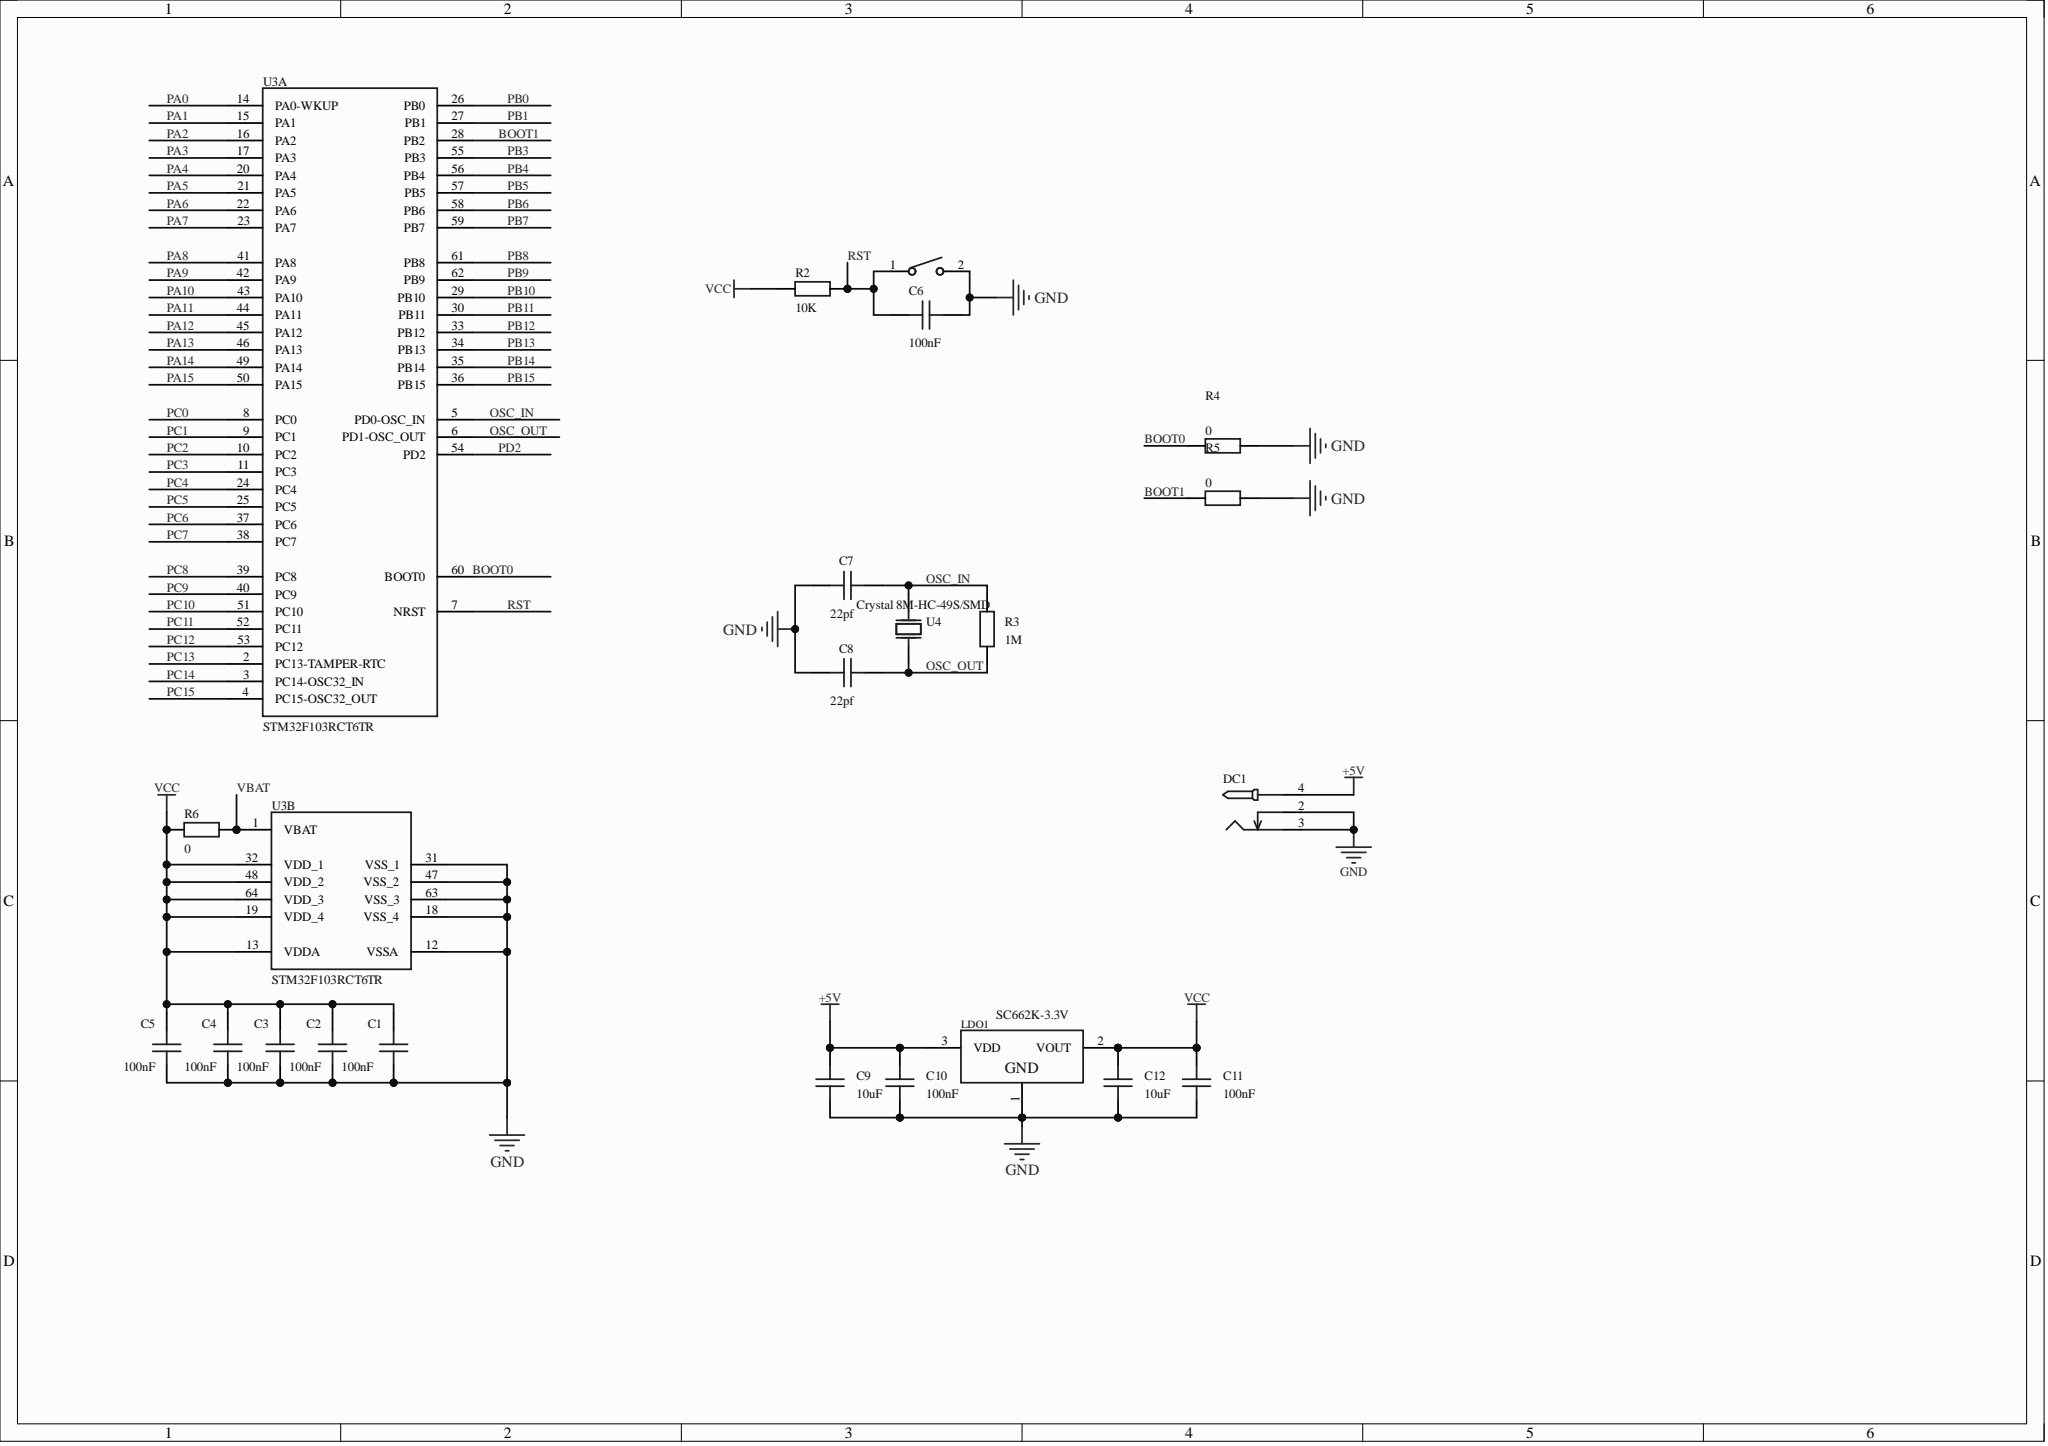Circuit board | Altium Designer | 22 parts | 9 nets
Bill of materials:
Comment,Description,Designator,Footprint,LibRef,Quantity
"100nF","[NoValue], Capacitance:100nF;Tolerance:±10%;Rated voltage:50V;Dielectric (temp. coefficient):X7R;","C1, C2, C3, C4, C5, C6, C10, C11","C0603","CAP_0603, CC0603KRX7R9BB104","8"
"22pf","","C7, C8","C0603","CAP_0603","2"
"10uF","Capacitance:10uF;Tolerance:±10%;Rated voltage:10V;Dielectric (temp. coefficient):X5R;","C9, C12","C0603","CL10A106KP8NNNC","2"
"","","DC1","DC-2.0","DC-005_2.0","1"
"SC662K-3.3V","Output type:Fixed;Output polarity:Positive;Max input voltage:6V;Output voltage:3.3V;Output current:250mA;Power supply ripple rejection (PSRR):50dB@(1kHz);","LDO1","SOT-23-3_L2.9-W1.3-P1.90-LS2.4-BR","SC662K-3.3V","1"
"10K","","R2","R0603","Res_0603","1"
"1M","","R3","R0603","Res_0603","1"
"0","","R4, R5, R6","R0603","Res_0603","3"
"SMD push button ANJIAN_2PIN","","SW1","SW-SMD_L6.0-W3.6-LS8.0","贴片按键ANJIAN_2PIN","1"
"STM32F103RCT6TR","CPU core:ARM Cortex-M3;Max CPU frequency:72MHz;Program storage capacity:256KB;Program memory type:FLASH;Total RAM:48KB;GPIO ports:51;","U3","LQFP-64_L10.0-W10.0-P0.50-LS12.0-BL","STM32F103RCT6TR","1"
"Crystal 8M-HC-49S/SMD","","U4","HC-49S_L11.4-W4.8-LS12.7","晶振8M-HC-49S/SMD","1"
Netlist (Protel format):
[
C1
C0603
100nF



]
[
C2
C0603
100nF



]
[
C3
C0603
100nF



]
[
C4
C0603
100nF



]
[
C5
C0603
100nF



]
[
C6
C0603
100nF



]
[
C7
C0603
22pf



]
[
C8
C0603
22pf



]
[
C9
C0603
10uF



]
[
C10
C0603
100nF



]
[
C11
C0603
100nF



]
[
C12
C0603
10uF



]
[
DC1
DC-2.0




]
[
LDO1
SOT-23-3_L2.9-W1.3-P1.90-LS2.4-BR
SC662K-3.3V



]
[
R2
R0603
10K



]
[
R3
R0603
1M



]
[
R4
R0603
0



]
[
R5
R0603
0



]
[
R6
R0603
0



]
[
SW1
SW-SMD_L6.0-W3.6-LS8.0
SMD push button ANJIAN_2PIN



]
[
U3
LQFP-64_L10.0-W10.0-P0.50-LS12.0-BL
STM32F103RCT6TR



]
[
U4
HC-49S_L11.4-W4.8-LS12.7
Crystal 8M-HC-49S/SMD



]
(
VCC
C1-1
C2-1
C3-1
C4-1
C5-1
C11-2
C12-2
LDO1-2
R2-1
R6-1
U3-13
U3-19
U3-32
U3-48
U3-64
)
(
VBAT
R6-2
U3-1
)
(
RST
C6-1
R2-2
SW1-1
U3-7
)
(
OSC_OUT
C8-2
R3-1
U3-6
U4-2
)
(
OSC_IN
C7-2
R3-2
U3-5
U4-1
)
(
GND
C1-2
C2-2
C3-2
C4-2
C5-2
C6-2
C7-1
C8-1
C9-1
C10-1
C11-1
C12-1
DC1-2
DC1-3
LDO1-1
R4-2
R5-2
SW1-2
U3-12
U3-18
U3-31
U3-47
U3-63
)
(
BOOT1
R5-1
U3-28
)
(
BOOT0
R4-1
U3-60
)
(
+5V
C9-2
C10-2
DC1-4
LDO1-3
)